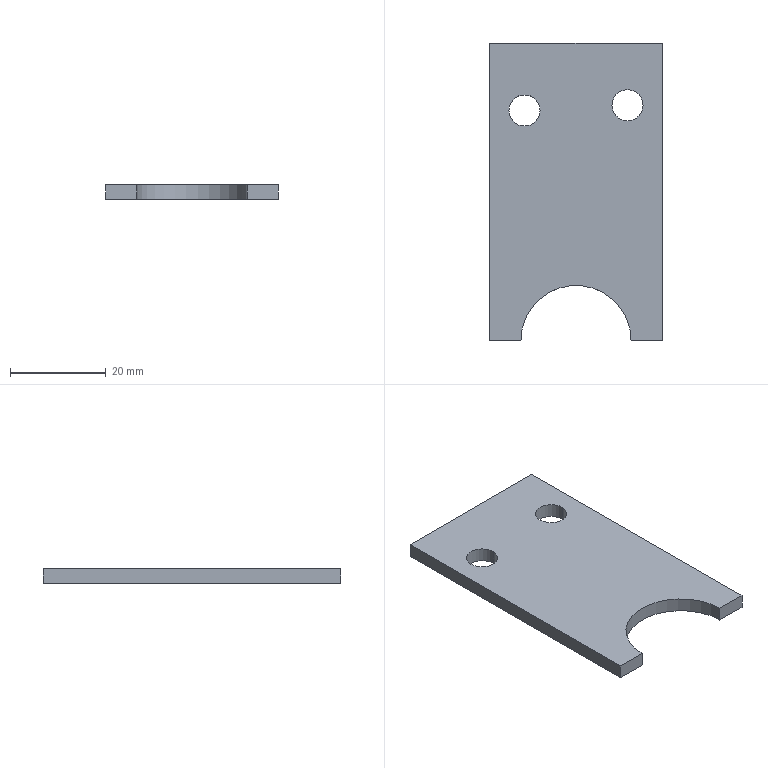Part | STEP file | 601-07-0070 | 1 solid | 12 faces | box 36 x 62 x 3 mm | volume 5874 mm3 | plane 7 | cylinder 5 | commonest cylinder face diameters 6.5 x4 23 x1
STEP:
#1=CARTESIAN_POINT('',(0.,0.,0.));
#2=DIRECTION('',(0.,0.,1.));
#3=DIRECTION('',(1.,0.,0.));
#4=AXIS2_PLACEMENT_3D('',#1,#2,#3);
#5=CARTESIAN_POINT('',(25.5,49.108,3.));
#6=VERTEX_POINT('',#5);
#7=CARTESIAN_POINT('',(25.5,49.108,0.));
#8=VERTEX_POINT('',#7);
#9=CARTESIAN_POINT('',(25.5,49.108,3.));
#10=DIRECTION('',(0.,0.,-1.));
#11=VECTOR('',#10,1.);
#12=LINE('',#9,#11);
#13=CARTESIAN_POINT('',(28.75,49.108,3.));
#14=DIRECTION('',(0.,0.,-1.));
#15=DIRECTION('',(-1.,0.,0.));
#16=AXIS2_PLACEMENT_3D('',#13,#14,#15);
#17=CYLINDRICAL_SURFACE('',#16,3.25);
#18=CARTESIAN_POINT('',(6.283,0.));
#19=DIRECTION('',(0.,1.));
#20=VECTOR('',#19,1.);
#21=LINE('',#18,#20);
#22=(GEOMETRIC_REPRESENTATION_CONTEXT(2)PARAMETRIC_REPRESENTATION_CONTEXT()REPRESENTATION_CONTEXT('',''));
#23=DEFINITIONAL_REPRESENTATION('',(#21),#22);
#24=PCURVE('',#17,#23);
#25=CARTESIAN_POINT('',(28.75,49.108,3.));
#26=DIRECTION('',(0.,0.,-1.));
#27=DIRECTION('',(-1.,0.,0.));
#28=AXIS2_PLACEMENT_3D('',#25,#26,#27);
#29=CYLINDRICAL_SURFACE('',#28,3.25);
#30=CARTESIAN_POINT('',(0.,0.));
#31=DIRECTION('',(0.,1.));
#32=VECTOR('',#31,1.);
#33=LINE('',#30,#32);
#34=(GEOMETRIC_REPRESENTATION_CONTEXT(2)PARAMETRIC_REPRESENTATION_CONTEXT()REPRESENTATION_CONTEXT('',''));
#35=DEFINITIONAL_REPRESENTATION('',(#33),#34);
#36=PCURVE('',#29,#35);
#37=SURFACE_CURVE('',#12,(#24,#36),.PCURVE_S1.);
#38=EDGE_CURVE('',#6,#8,#37,.T.);
#39=ORIENTED_EDGE('',*,*,#38,.T.);
#40=CARTESIAN_POINT('',(32.,49.108,0.));
#41=VERTEX_POINT('',#40);
#42=CARTESIAN_POINT('',(28.75,49.108,0.));
#43=DIRECTION('',(0.,0.,1.));
#44=DIRECTION('',(1.,0.,0.));
#45=AXIS2_PLACEMENT_3D('',#42,#43,#44);
#46=CIRCLE('',#45,3.25);
#47=CARTESIAN_POINT('',(9.425,3.));
#48=DIRECTION('',(-1.,0.));
#49=VECTOR('',#48,1.);
#50=LINE('',#47,#49);
#51=(GEOMETRIC_REPRESENTATION_CONTEXT(2)PARAMETRIC_REPRESENTATION_CONTEXT()REPRESENTATION_CONTEXT('',''));
#52=DEFINITIONAL_REPRESENTATION('',(#50),#51);
#53=PCURVE('',#17,#52);
#54=CARTESIAN_POINT('',(18.,0.,0.));
#55=DIRECTION('',(0.,0.,1.));
#56=DIRECTION('',(1.,0.,0.));
#57=AXIS2_PLACEMENT_3D('',#54,#55,#56);
#58=PLANE('',#57);
#59=CARTESIAN_POINT('',(10.75,49.108));
#60=DIRECTION('',(1.,0.));
#61=AXIS2_PLACEMENT_2D('',#59,#60);
#62=CIRCLE('',#61,3.25);
#63=(GEOMETRIC_REPRESENTATION_CONTEXT(2)PARAMETRIC_REPRESENTATION_CONTEXT()REPRESENTATION_CONTEXT('',''));
#64=DEFINITIONAL_REPRESENTATION('',(#62),#63);
#65=PCURVE('',#58,#64);
#66=SURFACE_CURVE('',#46,(#53,#65),.PCURVE_S1.);
#67=EDGE_CURVE('',#8,#41,#66,.T.);
#68=ORIENTED_EDGE('',*,*,#67,.T.);
#69=CARTESIAN_POINT('',(32.,49.108,3.));
#70=VERTEX_POINT('',#69);
#71=CARTESIAN_POINT('',(32.,49.108,3.));
#72=DIRECTION('',(0.,0.,-1.));
#73=VECTOR('',#72,1.);
#74=LINE('',#71,#73);
#75=CARTESIAN_POINT('',(3.142,0.));
#76=DIRECTION('',(0.,1.));
#77=VECTOR('',#76,1.);
#78=LINE('',#75,#77);
#79=(GEOMETRIC_REPRESENTATION_CONTEXT(2)PARAMETRIC_REPRESENTATION_CONTEXT()REPRESENTATION_CONTEXT('',''));
#80=DEFINITIONAL_REPRESENTATION('',(#78),#79);
#81=PCURVE('',#17,#80);
#82=CARTESIAN_POINT('',(3.142,0.));
#83=DIRECTION('',(0.,1.));
#84=VECTOR('',#83,1.);
#85=LINE('',#82,#84);
#86=(GEOMETRIC_REPRESENTATION_CONTEXT(2)PARAMETRIC_REPRESENTATION_CONTEXT()REPRESENTATION_CONTEXT('',''));
#87=DEFINITIONAL_REPRESENTATION('',(#85),#86);
#88=PCURVE('',#29,#87);
#89=SURFACE_CURVE('',#74,(#81,#88),.PCURVE_S1.);
#90=EDGE_CURVE('',#70,#41,#89,.T.);
#91=ORIENTED_EDGE('',*,*,#90,.F.);
#92=CARTESIAN_POINT('',(28.75,49.108,3.));
#93=DIRECTION('',(0.,0.,1.));
#94=DIRECTION('',(1.,0.,0.));
#95=AXIS2_PLACEMENT_3D('',#92,#93,#94);
#96=CIRCLE('',#95,3.25);
#97=CARTESIAN_POINT('',(9.425,0.));
#98=DIRECTION('',(-1.,0.));
#99=VECTOR('',#98,1.);
#100=LINE('',#97,#99);
#101=(GEOMETRIC_REPRESENTATION_CONTEXT(2)PARAMETRIC_REPRESENTATION_CONTEXT()REPRESENTATION_CONTEXT('',''));
#102=DEFINITIONAL_REPRESENTATION('',(#100),#101);
#103=PCURVE('',#17,#102);
#104=CARTESIAN_POINT('',(18.,0.,3.));
#105=DIRECTION('',(0.,0.,1.));
#106=DIRECTION('',(1.,0.,0.));
#107=AXIS2_PLACEMENT_3D('',#104,#105,#106);
#108=PLANE('',#107);
#109=CARTESIAN_POINT('',(10.75,49.108));
#110=DIRECTION('',(1.,0.));
#111=AXIS2_PLACEMENT_2D('',#109,#110);
#112=CIRCLE('',#111,3.25);
#113=(GEOMETRIC_REPRESENTATION_CONTEXT(2)PARAMETRIC_REPRESENTATION_CONTEXT()REPRESENTATION_CONTEXT('',''));
#114=DEFINITIONAL_REPRESENTATION('',(#112),#113);
#115=PCURVE('',#108,#114);
#116=SURFACE_CURVE('',#96,(#103,#115),.PCURVE_S1.);
#117=EDGE_CURVE('',#6,#70,#116,.T.);
#118=ORIENTED_EDGE('',*,*,#117,.F.);
#119=EDGE_LOOP('',(#39,#68,#91,#118));
#120=FACE_BOUND('',#119,.F.);
#121=ADVANCED_FACE('',(#120),#17,.F.);
#122=CARTESIAN_POINT('',(4.,48.,3.));
#123=VERTEX_POINT('',#122);
#124=CARTESIAN_POINT('',(4.,48.,0.));
#125=VERTEX_POINT('',#124);
#126=CARTESIAN_POINT('',(4.,48.,3.));
#127=DIRECTION('',(0.,0.,-1.));
#128=VECTOR('',#127,1.);
#129=LINE('',#126,#128);
#130=CARTESIAN_POINT('',(7.25,48.,3.));
#131=DIRECTION('',(0.,0.,-1.));
#132=DIRECTION('',(-1.,0.,0.));
#133=AXIS2_PLACEMENT_3D('',#130,#131,#132);
#134=CYLINDRICAL_SURFACE('',#133,3.25);
#135=CARTESIAN_POINT('',(6.283,0.));
#136=DIRECTION('',(0.,1.));
#137=VECTOR('',#136,1.);
#138=LINE('',#135,#137);
#139=(GEOMETRIC_REPRESENTATION_CONTEXT(2)PARAMETRIC_REPRESENTATION_CONTEXT()REPRESENTATION_CONTEXT('',''));
#140=DEFINITIONAL_REPRESENTATION('',(#138),#139);
#141=PCURVE('',#134,#140);
#142=CARTESIAN_POINT('',(7.25,48.,3.));
#143=DIRECTION('',(0.,0.,-1.));
#144=DIRECTION('',(-1.,0.,0.));
#145=AXIS2_PLACEMENT_3D('',#142,#143,#144);
#146=CYLINDRICAL_SURFACE('',#145,3.25);
#147=CARTESIAN_POINT('',(0.,0.));
#148=DIRECTION('',(0.,1.));
#149=VECTOR('',#148,1.);
#150=LINE('',#147,#149);
#151=(GEOMETRIC_REPRESENTATION_CONTEXT(2)PARAMETRIC_REPRESENTATION_CONTEXT()REPRESENTATION_CONTEXT('',''));
#152=DEFINITIONAL_REPRESENTATION('',(#150),#151);
#153=PCURVE('',#146,#152);
#154=SURFACE_CURVE('',#129,(#141,#153),.PCURVE_S1.);
#155=EDGE_CURVE('',#123,#125,#154,.T.);
#156=ORIENTED_EDGE('',*,*,#155,.T.);
#157=CARTESIAN_POINT('',(10.5,48.,0.));
#158=VERTEX_POINT('',#157);
#159=CARTESIAN_POINT('',(7.25,48.,0.));
#160=DIRECTION('',(0.,0.,1.));
#161=DIRECTION('',(1.,0.,0.));
#162=AXIS2_PLACEMENT_3D('',#159,#160,#161);
#163=CIRCLE('',#162,3.25);
#164=CARTESIAN_POINT('',(9.425,3.));
#165=DIRECTION('',(-1.,0.));
#166=VECTOR('',#165,1.);
#167=LINE('',#164,#166);
#168=(GEOMETRIC_REPRESENTATION_CONTEXT(2)PARAMETRIC_REPRESENTATION_CONTEXT()REPRESENTATION_CONTEXT('',''));
#169=DEFINITIONAL_REPRESENTATION('',(#167),#168);
#170=PCURVE('',#134,#169);
#171=CARTESIAN_POINT('',(-10.75,48.));
#172=DIRECTION('',(1.,0.));
#173=AXIS2_PLACEMENT_2D('',#171,#172);
#174=CIRCLE('',#173,3.25);
#175=(GEOMETRIC_REPRESENTATION_CONTEXT(2)PARAMETRIC_REPRESENTATION_CONTEXT()REPRESENTATION_CONTEXT('',''));
#176=DEFINITIONAL_REPRESENTATION('',(#174),#175);
#177=PCURVE('',#58,#176);
#178=SURFACE_CURVE('',#163,(#170,#177),.PCURVE_S1.);
#179=EDGE_CURVE('',#125,#158,#178,.T.);
#180=ORIENTED_EDGE('',*,*,#179,.T.);
#181=CARTESIAN_POINT('',(10.5,48.,3.));
#182=VERTEX_POINT('',#181);
#183=CARTESIAN_POINT('',(10.5,48.,3.));
#184=DIRECTION('',(0.,0.,-1.));
#185=VECTOR('',#184,1.);
#186=LINE('',#183,#185);
#187=CARTESIAN_POINT('',(3.142,0.));
#188=DIRECTION('',(0.,1.));
#189=VECTOR('',#188,1.);
#190=LINE('',#187,#189);
#191=(GEOMETRIC_REPRESENTATION_CONTEXT(2)PARAMETRIC_REPRESENTATION_CONTEXT()REPRESENTATION_CONTEXT('',''));
#192=DEFINITIONAL_REPRESENTATION('',(#190),#191);
#193=PCURVE('',#134,#192);
#194=CARTESIAN_POINT('',(3.142,0.));
#195=DIRECTION('',(0.,1.));
#196=VECTOR('',#195,1.);
#197=LINE('',#194,#196);
#198=(GEOMETRIC_REPRESENTATION_CONTEXT(2)PARAMETRIC_REPRESENTATION_CONTEXT()REPRESENTATION_CONTEXT('',''));
#199=DEFINITIONAL_REPRESENTATION('',(#197),#198);
#200=PCURVE('',#146,#199);
#201=SURFACE_CURVE('',#186,(#193,#200),.PCURVE_S1.);
#202=EDGE_CURVE('',#182,#158,#201,.T.);
#203=ORIENTED_EDGE('',*,*,#202,.F.);
#204=CARTESIAN_POINT('',(7.25,48.,3.));
#205=DIRECTION('',(0.,0.,1.));
#206=DIRECTION('',(1.,0.,0.));
#207=AXIS2_PLACEMENT_3D('',#204,#205,#206);
#208=CIRCLE('',#207,3.25);
#209=CARTESIAN_POINT('',(9.425,0.));
#210=DIRECTION('',(-1.,0.));
#211=VECTOR('',#210,1.);
#212=LINE('',#209,#211);
#213=(GEOMETRIC_REPRESENTATION_CONTEXT(2)PARAMETRIC_REPRESENTATION_CONTEXT()REPRESENTATION_CONTEXT('',''));
#214=DEFINITIONAL_REPRESENTATION('',(#212),#213);
#215=PCURVE('',#134,#214);
#216=CARTESIAN_POINT('',(-10.75,48.));
#217=DIRECTION('',(1.,0.));
#218=AXIS2_PLACEMENT_2D('',#216,#217);
#219=CIRCLE('',#218,3.25);
#220=(GEOMETRIC_REPRESENTATION_CONTEXT(2)PARAMETRIC_REPRESENTATION_CONTEXT()REPRESENTATION_CONTEXT('',''));
#221=DEFINITIONAL_REPRESENTATION('',(#219),#220);
#222=PCURVE('',#108,#221);
#223=SURFACE_CURVE('',#208,(#215,#222),.PCURVE_S1.);
#224=EDGE_CURVE('',#123,#182,#223,.T.);
#225=ORIENTED_EDGE('',*,*,#224,.F.);
#226=EDGE_LOOP('',(#156,#180,#203,#225));
#227=FACE_BOUND('',#226,.F.);
#228=ADVANCED_FACE('',(#227),#134,.F.);
#229=ORIENTED_EDGE('',*,*,#224,.F.);
#230=CARTESIAN_POINT('',(7.25,48.,3.));
#231=DIRECTION('',(0.,0.,1.));
#232=DIRECTION('',(1.,0.,0.));
#233=AXIS2_PLACEMENT_3D('',#230,#231,#232);
#234=CIRCLE('',#233,3.25);
#235=CARTESIAN_POINT('',(-10.75,48.));
#236=DIRECTION('',(1.,0.));
#237=AXIS2_PLACEMENT_2D('',#235,#236);
#238=CIRCLE('',#237,3.25);
#239=(GEOMETRIC_REPRESENTATION_CONTEXT(2)PARAMETRIC_REPRESENTATION_CONTEXT()REPRESENTATION_CONTEXT('',''));
#240=DEFINITIONAL_REPRESENTATION('',(#238),#239);
#241=PCURVE('',#108,#240);
#242=CARTESIAN_POINT('',(3.142,0.));
#243=DIRECTION('',(-1.,0.));
#244=VECTOR('',#243,1.);
#245=LINE('',#242,#244);
#246=(GEOMETRIC_REPRESENTATION_CONTEXT(2)PARAMETRIC_REPRESENTATION_CONTEXT()REPRESENTATION_CONTEXT('',''));
#247=DEFINITIONAL_REPRESENTATION('',(#245),#246);
#248=PCURVE('',#146,#247);
#249=SURFACE_CURVE('',#234,(#241,#248),.PCURVE_S1.);
#250=EDGE_CURVE('',#182,#123,#249,.T.);
#251=ORIENTED_EDGE('',*,*,#250,.F.);
#252=EDGE_LOOP('',(#229,#251));
#253=FACE_BOUND('',#252,.T.);
#254=CARTESIAN_POINT('',(0.,62.,3.));
#255=VERTEX_POINT('',#254);
#256=CARTESIAN_POINT('',(0.,0.,3.));
#257=VERTEX_POINT('',#256);
#258=CARTESIAN_POINT('',(0.,0.,3.));
#259=DIRECTION('',(0.,-1.,0.));
#260=VECTOR('',#259,1.);
#261=LINE('',#258,#260);
#262=CARTESIAN_POINT('',(-18.,0.));
#263=DIRECTION('',(0.,-1.));
#264=VECTOR('',#263,1.);
#265=LINE('',#262,#264);
#266=(GEOMETRIC_REPRESENTATION_CONTEXT(2)PARAMETRIC_REPRESENTATION_CONTEXT()REPRESENTATION_CONTEXT('',''));
#267=DEFINITIONAL_REPRESENTATION('',(#265),#266);
#268=PCURVE('',#108,#267);
#269=CARTESIAN_POINT('',(0.,0.,3.));
#270=DIRECTION('',(1.,0.,0.));
#271=DIRECTION('',(0.,1.,0.));
#272=AXIS2_PLACEMENT_3D('',#269,#270,#271);
#273=PLANE('',#272);
#274=CARTESIAN_POINT('',(0.,0.));
#275=DIRECTION('',(-1.,0.));
#276=VECTOR('',#275,1.);
#277=LINE('',#274,#276);
#278=(GEOMETRIC_REPRESENTATION_CONTEXT(2)PARAMETRIC_REPRESENTATION_CONTEXT()REPRESENTATION_CONTEXT('',''));
#279=DEFINITIONAL_REPRESENTATION('',(#277),#278);
#280=PCURVE('',#273,#279);
#281=SURFACE_CURVE('',#261,(#268,#280),.PCURVE_S1.);
#282=EDGE_CURVE('',#255,#257,#281,.T.);
#283=ORIENTED_EDGE('',*,*,#282,.T.);
#284=CARTESIAN_POINT('',(6.5,0.,3.));
#285=VERTEX_POINT('',#284);
#286=CARTESIAN_POINT('',(0.,0.,3.));
#287=DIRECTION('',(1.,0.,0.));
#288=VECTOR('',#287,1.);
#289=LINE('',#286,#288);
#290=CARTESIAN_POINT('',(-18.,0.));
#291=DIRECTION('',(1.,0.));
#292=VECTOR('',#291,1.);
#293=LINE('',#290,#292);
#294=(GEOMETRIC_REPRESENTATION_CONTEXT(2)PARAMETRIC_REPRESENTATION_CONTEXT()REPRESENTATION_CONTEXT('',''));
#295=DEFINITIONAL_REPRESENTATION('',(#293),#294);
#296=PCURVE('',#108,#295);
#297=CARTESIAN_POINT('',(0.,0.,3.));
#298=DIRECTION('',(0.,1.,0.));
#299=DIRECTION('',(0.,0.,1.));
#300=AXIS2_PLACEMENT_3D('',#297,#298,#299);
#301=PLANE('',#300);
#302=CARTESIAN_POINT('',(0.,0.));
#303=DIRECTION('',(0.,1.));
#304=VECTOR('',#303,1.);
#305=LINE('',#302,#304);
#306=(GEOMETRIC_REPRESENTATION_CONTEXT(2)PARAMETRIC_REPRESENTATION_CONTEXT()REPRESENTATION_CONTEXT('',''));
#307=DEFINITIONAL_REPRESENTATION('',(#305),#306);
#308=PCURVE('',#301,#307);
#309=SURFACE_CURVE('',#289,(#296,#308),.PCURVE_S1.);
#310=EDGE_CURVE('',#257,#285,#309,.T.);
#311=ORIENTED_EDGE('',*,*,#310,.T.);
#312=CARTESIAN_POINT('',(29.5,0.,3.));
#313=VERTEX_POINT('',#312);
#314=CARTESIAN_POINT('',(18.,0.,3.));
#315=DIRECTION('',(0.,0.,-1.));
#316=DIRECTION('',(1.,0.,0.));
#317=AXIS2_PLACEMENT_3D('',#314,#315,#316);
#318=CIRCLE('',#317,11.5);
#319=CARTESIAN_POINT('',(11.5,0.));
#320=CARTESIAN_POINT('',(11.5,-19.919));
#321=CARTESIAN_POINT('',(-5.75,-9.959));
#322=CARTESIAN_POINT('',(-23.,0.));
#323=CARTESIAN_POINT('',(-5.75,9.959));
#324=CARTESIAN_POINT('',(11.5,19.919));
#325=CARTESIAN_POINT('',(11.5,0.));
#326=(BOUNDED_CURVE()B_SPLINE_CURVE(2,(#319,#320,#321,#322,#323,#324,#325),.UNSPECIFIED.,.T.,.F.)B_SPLINE_CURVE_WITH_KNOTS((1,2,2,2,2,1),(-2.094,0.,2.094,4.189,6.283,8.378),.UNSPECIFIED.)CURVE()GEOMETRIC_REPRESENTATION_ITEM()RATIONAL_B_SPLINE_CURVE((1.,0.5,1.,0.5,1.,0.5,1.))REPRESENTATION_ITEM(''));
#327=(GEOMETRIC_REPRESENTATION_CONTEXT(2)PARAMETRIC_REPRESENTATION_CONTEXT()REPRESENTATION_CONTEXT('',''));
#328=DEFINITIONAL_REPRESENTATION('',(#326),#327);
#329=PCURVE('',#108,#328);
#330=CARTESIAN_POINT('',(18.,0.,3.));
#331=DIRECTION('',(0.,0.,-1.));
#332=DIRECTION('',(-1.,0.,0.));
#333=AXIS2_PLACEMENT_3D('',#330,#331,#332);
#334=CYLINDRICAL_SURFACE('',#333,11.5);
#335=CARTESIAN_POINT('',(-3.142,0.));
#336=DIRECTION('',(1.,0.));
#337=VECTOR('',#336,1.);
#338=LINE('',#335,#337);
#339=(GEOMETRIC_REPRESENTATION_CONTEXT(2)PARAMETRIC_REPRESENTATION_CONTEXT()REPRESENTATION_CONTEXT('',''));
#340=DEFINITIONAL_REPRESENTATION('',(#338),#339);
#341=PCURVE('',#334,#340);
#342=SURFACE_CURVE('',#318,(#329,#341),.PCURVE_S1.);
#343=EDGE_CURVE('',#285,#313,#342,.T.);
#344=ORIENTED_EDGE('',*,*,#343,.T.);
#345=CARTESIAN_POINT('',(36.,0.,3.));
#346=VERTEX_POINT('',#345);
#347=CARTESIAN_POINT('',(29.5,0.,3.));
#348=DIRECTION('',(1.,0.,0.));
#349=VECTOR('',#348,1.);
#350=LINE('',#347,#349);
#351=CARTESIAN_POINT('',(11.5,0.));
#352=DIRECTION('',(1.,0.));
#353=VECTOR('',#352,1.);
#354=LINE('',#351,#353);
#355=(GEOMETRIC_REPRESENTATION_CONTEXT(2)PARAMETRIC_REPRESENTATION_CONTEXT()REPRESENTATION_CONTEXT('',''));
#356=DEFINITIONAL_REPRESENTATION('',(#354),#355);
#357=PCURVE('',#108,#356);
#358=CARTESIAN_POINT('',(29.5,0.,3.));
#359=DIRECTION('',(0.,1.,0.));
#360=DIRECTION('',(0.,0.,1.));
#361=AXIS2_PLACEMENT_3D('',#358,#359,#360);
#362=PLANE('',#361);
#363=CARTESIAN_POINT('',(0.,0.));
#364=DIRECTION('',(0.,1.));
#365=VECTOR('',#364,1.);
#366=LINE('',#363,#365);
#367=(GEOMETRIC_REPRESENTATION_CONTEXT(2)PARAMETRIC_REPRESENTATION_CONTEXT()REPRESENTATION_CONTEXT('',''));
#368=DEFINITIONAL_REPRESENTATION('',(#366),#367);
#369=PCURVE('',#362,#368);
#370=SURFACE_CURVE('',#350,(#357,#369),.PCURVE_S1.);
#371=EDGE_CURVE('',#313,#346,#370,.T.);
#372=ORIENTED_EDGE('',*,*,#371,.T.);
#373=CARTESIAN_POINT('',(36.,62.,3.));
#374=VERTEX_POINT('',#373);
#375=CARTESIAN_POINT('',(36.,0.,3.));
#376=DIRECTION('',(0.,1.,0.));
#377=VECTOR('',#376,1.);
#378=LINE('',#375,#377);
#379=CARTESIAN_POINT('',(18.,0.));
#380=DIRECTION('',(0.,1.));
#381=VECTOR('',#380,1.);
#382=LINE('',#379,#381);
#383=(GEOMETRIC_REPRESENTATION_CONTEXT(2)PARAMETRIC_REPRESENTATION_CONTEXT()REPRESENTATION_CONTEXT('',''));
#384=DEFINITIONAL_REPRESENTATION('',(#382),#383);
#385=PCURVE('',#108,#384);
#386=CARTESIAN_POINT('',(36.,0.,3.));
#387=DIRECTION('',(-1.,0.,0.));
#388=DIRECTION('',(0.,-1.,0.));
#389=AXIS2_PLACEMENT_3D('',#386,#387,#388);
#390=PLANE('',#389);
#391=CARTESIAN_POINT('',(0.,0.));
#392=DIRECTION('',(-1.,0.));
#393=VECTOR('',#392,1.);
#394=LINE('',#391,#393);
#395=(GEOMETRIC_REPRESENTATION_CONTEXT(2)PARAMETRIC_REPRESENTATION_CONTEXT()REPRESENTATION_CONTEXT('',''));
#396=DEFINITIONAL_REPRESENTATION('',(#394),#395);
#397=PCURVE('',#390,#396);
#398=SURFACE_CURVE('',#378,(#385,#397),.PCURVE_S1.);
#399=EDGE_CURVE('',#346,#374,#398,.T.);
#400=ORIENTED_EDGE('',*,*,#399,.T.);
#401=CARTESIAN_POINT('',(0.,62.,3.));
#402=DIRECTION('',(-1.,0.,0.));
#403=VECTOR('',#402,1.);
#404=LINE('',#401,#403);
#405=CARTESIAN_POINT('',(-18.,62.));
#406=DIRECTION('',(-1.,0.));
#407=VECTOR('',#406,1.);
#408=LINE('',#405,#407);
#409=(GEOMETRIC_REPRESENTATION_CONTEXT(2)PARAMETRIC_REPRESENTATION_CONTEXT()REPRESENTATION_CONTEXT('',''));
#410=DEFINITIONAL_REPRESENTATION('',(#408),#409);
#411=PCURVE('',#108,#410);
#412=CARTESIAN_POINT('',(0.,62.,3.));
#413=DIRECTION('',(0.,-1.,0.));
#414=DIRECTION('',(0.,0.,-1.));
#415=AXIS2_PLACEMENT_3D('',#412,#413,#414);
#416=PLANE('',#415);
#417=CARTESIAN_POINT('',(0.,0.));
#418=DIRECTION('',(0.,-1.));
#419=VECTOR('',#418,1.);
#420=LINE('',#417,#419);
#421=(GEOMETRIC_REPRESENTATION_CONTEXT(2)PARAMETRIC_REPRESENTATION_CONTEXT()REPRESENTATION_CONTEXT('',''));
#422=DEFINITIONAL_REPRESENTATION('',(#420),#421);
#423=PCURVE('',#416,#422);
#424=SURFACE_CURVE('',#404,(#411,#423),.PCURVE_S1.);
#425=EDGE_CURVE('',#374,#255,#424,.T.);
#426=ORIENTED_EDGE('',*,*,#425,.T.);
#427=EDGE_LOOP('',(#283,#311,#344,#372,#400,#426));
#428=FACE_BOUND('',#427,.T.);
#429=ORIENTED_EDGE('',*,*,#117,.F.);
#430=CARTESIAN_POINT('',(28.75,49.108,3.));
#431=DIRECTION('',(0.,0.,1.));
#432=DIRECTION('',(1.,0.,0.));
#433=AXIS2_PLACEMENT_3D('',#430,#431,#432);
#434=CIRCLE('',#433,3.25);
#435=CARTESIAN_POINT('',(10.75,49.108));
#436=DIRECTION('',(1.,0.));
#437=AXIS2_PLACEMENT_2D('',#435,#436);
#438=CIRCLE('',#437,3.25);
#439=(GEOMETRIC_REPRESENTATION_CONTEXT(2)PARAMETRIC_REPRESENTATION_CONTEXT()REPRESENTATION_CONTEXT('',''));
#440=DEFINITIONAL_REPRESENTATION('',(#438),#439);
#441=PCURVE('',#108,#440);
#442=CARTESIAN_POINT('',(3.142,0.));
#443=DIRECTION('',(-1.,0.));
#444=VECTOR('',#443,1.);
#445=LINE('',#442,#444);
#446=(GEOMETRIC_REPRESENTATION_CONTEXT(2)PARAMETRIC_REPRESENTATION_CONTEXT()REPRESENTATION_CONTEXT('',''));
#447=DEFINITIONAL_REPRESENTATION('',(#445),#446);
#448=PCURVE('',#29,#447);
#449=SURFACE_CURVE('',#434,(#441,#448),.PCURVE_S1.);
#450=EDGE_CURVE('',#70,#6,#449,.T.);
#451=ORIENTED_EDGE('',*,*,#450,.F.);
#452=EDGE_LOOP('',(#429,#451));
#453=FACE_BOUND('',#452,.T.);
#454=ADVANCED_FACE('',(#253,#428,#453),#108,.T.);
#455=ORIENTED_EDGE('',*,*,#179,.T.);
#456=CARTESIAN_POINT('',(7.25,48.,0.));
#457=DIRECTION('',(0.,0.,1.));
#458=DIRECTION('',(1.,0.,0.));
#459=AXIS2_PLACEMENT_3D('',#456,#457,#458);
#460=CIRCLE('',#459,3.25);
#461=CARTESIAN_POINT('',(-10.75,48.));
#462=DIRECTION('',(1.,0.));
#463=AXIS2_PLACEMENT_2D('',#461,#462);
#464=CIRCLE('',#463,3.25);
#465=(GEOMETRIC_REPRESENTATION_CONTEXT(2)PARAMETRIC_REPRESENTATION_CONTEXT()REPRESENTATION_CONTEXT('',''));
#466=DEFINITIONAL_REPRESENTATION('',(#464),#465);
#467=PCURVE('',#58,#466);
#468=CARTESIAN_POINT('',(3.142,3.));
#469=DIRECTION('',(-1.,0.));
#470=VECTOR('',#469,1.);
#471=LINE('',#468,#470);
#472=(GEOMETRIC_REPRESENTATION_CONTEXT(2)PARAMETRIC_REPRESENTATION_CONTEXT()REPRESENTATION_CONTEXT('',''));
#473=DEFINITIONAL_REPRESENTATION('',(#471),#472);
#474=PCURVE('',#146,#473);
#475=SURFACE_CURVE('',#460,(#467,#474),.PCURVE_S1.);
#476=EDGE_CURVE('',#158,#125,#475,.T.);
#477=ORIENTED_EDGE('',*,*,#476,.T.);
#478=EDGE_LOOP('',(#455,#477));
#479=FACE_BOUND('',#478,.T.);
#480=CARTESIAN_POINT('',(0.,62.,0.));
#481=VERTEX_POINT('',#480);
#482=CARTESIAN_POINT('',(0.,0.,0.));
#483=VERTEX_POINT('',#482);
#484=CARTESIAN_POINT('',(0.,0.,0.));
#485=DIRECTION('',(0.,-1.,0.));
#486=VECTOR('',#485,1.);
#487=LINE('',#484,#486);
#488=CARTESIAN_POINT('',(-18.,0.));
#489=DIRECTION('',(0.,-1.));
#490=VECTOR('',#489,1.);
#491=LINE('',#488,#490);
#492=(GEOMETRIC_REPRESENTATION_CONTEXT(2)PARAMETRIC_REPRESENTATION_CONTEXT()REPRESENTATION_CONTEXT('',''));
#493=DEFINITIONAL_REPRESENTATION('',(#491),#492);
#494=PCURVE('',#58,#493);
#495=CARTESIAN_POINT('',(0.,-3.));
#496=DIRECTION('',(-1.,0.));
#497=VECTOR('',#496,1.);
#498=LINE('',#495,#497);
#499=(GEOMETRIC_REPRESENTATION_CONTEXT(2)PARAMETRIC_REPRESENTATION_CONTEXT()REPRESENTATION_CONTEXT('',''));
#500=DEFINITIONAL_REPRESENTATION('',(#498),#499);
#501=PCURVE('',#273,#500);
#502=SURFACE_CURVE('',#487,(#494,#501),.PCURVE_S1.);
#503=EDGE_CURVE('',#481,#483,#502,.T.);
#504=ORIENTED_EDGE('',*,*,#503,.F.);
#505=CARTESIAN_POINT('',(36.,62.,0.));
#506=VERTEX_POINT('',#505);
#507=CARTESIAN_POINT('',(0.,62.,0.));
#508=DIRECTION('',(-1.,0.,0.));
#509=VECTOR('',#508,1.);
#510=LINE('',#507,#509);
#511=CARTESIAN_POINT('',(-18.,62.));
#512=DIRECTION('',(-1.,0.));
#513=VECTOR('',#512,1.);
#514=LINE('',#511,#513);
#515=(GEOMETRIC_REPRESENTATION_CONTEXT(2)PARAMETRIC_REPRESENTATION_CONTEXT()REPRESENTATION_CONTEXT('',''));
#516=DEFINITIONAL_REPRESENTATION('',(#514),#515);
#517=PCURVE('',#58,#516);
#518=CARTESIAN_POINT('',(3.,0.));
#519=DIRECTION('',(0.,-1.));
#520=VECTOR('',#519,1.);
#521=LINE('',#518,#520);
#522=(GEOMETRIC_REPRESENTATION_CONTEXT(2)PARAMETRIC_REPRESENTATION_CONTEXT()REPRESENTATION_CONTEXT('',''));
#523=DEFINITIONAL_REPRESENTATION('',(#521),#522);
#524=PCURVE('',#416,#523);
#525=SURFACE_CURVE('',#510,(#517,#524),.PCURVE_S1.);
#526=EDGE_CURVE('',#506,#481,#525,.T.);
#527=ORIENTED_EDGE('',*,*,#526,.F.);
#528=CARTESIAN_POINT('',(36.,0.,0.));
#529=VERTEX_POINT('',#528);
#530=CARTESIAN_POINT('',(36.,0.,0.));
#531=DIRECTION('',(0.,1.,0.));
#532=VECTOR('',#531,1.);
#533=LINE('',#530,#532);
#534=CARTESIAN_POINT('',(18.,0.));
#535=DIRECTION('',(0.,1.));
#536=VECTOR('',#535,1.);
#537=LINE('',#534,#536);
#538=(GEOMETRIC_REPRESENTATION_CONTEXT(2)PARAMETRIC_REPRESENTATION_CONTEXT()REPRESENTATION_CONTEXT('',''));
#539=DEFINITIONAL_REPRESENTATION('',(#537),#538);
#540=PCURVE('',#58,#539);
#541=CARTESIAN_POINT('',(0.,-3.));
#542=DIRECTION('',(-1.,0.));
#543=VECTOR('',#542,1.);
#544=LINE('',#541,#543);
#545=(GEOMETRIC_REPRESENTATION_CONTEXT(2)PARAMETRIC_REPRESENTATION_CONTEXT()REPRESENTATION_CONTEXT('',''));
#546=DEFINITIONAL_REPRESENTATION('',(#544),#545);
#547=PCURVE('',#390,#546);
#548=SURFACE_CURVE('',#533,(#540,#547),.PCURVE_S1.);
#549=EDGE_CURVE('',#529,#506,#548,.T.);
#550=ORIENTED_EDGE('',*,*,#549,.F.);
#551=CARTESIAN_POINT('',(29.5,0.,0.));
#552=VERTEX_POINT('',#551);
#553=CARTESIAN_POINT('',(29.5,0.,0.));
#554=DIRECTION('',(1.,0.,0.));
#555=VECTOR('',#554,1.);
#556=LINE('',#553,#555);
#557=CARTESIAN_POINT('',(11.5,0.));
#558=DIRECTION('',(1.,0.));
#559=VECTOR('',#558,1.);
#560=LINE('',#557,#559);
#561=(GEOMETRIC_REPRESENTATION_CONTEXT(2)PARAMETRIC_REPRESENTATION_CONTEXT()REPRESENTATION_CONTEXT('',''));
#562=DEFINITIONAL_REPRESENTATION('',(#560),#561);
#563=PCURVE('',#58,#562);
#564=CARTESIAN_POINT('',(-3.,0.));
#565=DIRECTION('',(0.,1.));
#566=VECTOR('',#565,1.);
#567=LINE('',#564,#566);
#568=(GEOMETRIC_REPRESENTATION_CONTEXT(2)PARAMETRIC_REPRESENTATION_CONTEXT()REPRESENTATION_CONTEXT('',''));
#569=DEFINITIONAL_REPRESENTATION('',(#567),#568);
#570=PCURVE('',#362,#569);
#571=SURFACE_CURVE('',#556,(#563,#570),.PCURVE_S1.);
#572=EDGE_CURVE('',#552,#529,#571,.T.);
#573=ORIENTED_EDGE('',*,*,#572,.F.);
#574=CARTESIAN_POINT('',(6.5,0.,0.));
#575=VERTEX_POINT('',#574);
#576=CARTESIAN_POINT('',(18.,0.,0.));
#577=DIRECTION('',(0.,0.,-1.));
#578=DIRECTION('',(1.,0.,0.));
#579=AXIS2_PLACEMENT_3D('',#576,#577,#578);
#580=CIRCLE('',#579,11.5);
#581=CARTESIAN_POINT('',(11.5,0.));
#582=CARTESIAN_POINT('',(11.5,-19.919));
#583=CARTESIAN_POINT('',(-5.75,-9.959));
#584=CARTESIAN_POINT('',(-23.,0.));
#585=CARTESIAN_POINT('',(-5.75,9.959));
#586=CARTESIAN_POINT('',(11.5,19.919));
#587=CARTESIAN_POINT('',(11.5,0.));
#588=(BOUNDED_CURVE()B_SPLINE_CURVE(2,(#581,#582,#583,#584,#585,#586,#587),.UNSPECIFIED.,.T.,.F.)B_SPLINE_CURVE_WITH_KNOTS((1,2,2,2,2,1),(-2.094,0.,2.094,4.189,6.283,8.378),.UNSPECIFIED.)CURVE()GEOMETRIC_REPRESENTATION_ITEM()RATIONAL_B_SPLINE_CURVE((1.,0.5,1.,0.5,1.,0.5,1.))REPRESENTATION_ITEM(''));
#589=(GEOMETRIC_REPRESENTATION_CONTEXT(2)PARAMETRIC_REPRESENTATION_CONTEXT()REPRESENTATION_CONTEXT('',''));
#590=DEFINITIONAL_REPRESENTATION('',(#588),#589);
#591=PCURVE('',#58,#590);
#592=CARTESIAN_POINT('',(-3.142,3.));
#593=DIRECTION('',(1.,0.));
#594=VECTOR('',#593,1.);
#595=LINE('',#592,#594);
#596=(GEOMETRIC_REPRESENTATION_CONTEXT(2)PARAMETRIC_REPRESENTATION_CONTEXT()REPRESENTATION_CONTEXT('',''));
#597=DEFINITIONAL_REPRESENTATION('',(#595),#596);
#598=PCURVE('',#334,#597);
#599=SURFACE_CURVE('',#580,(#591,#598),.PCURVE_S1.);
#600=EDGE_CURVE('',#575,#552,#599,.T.);
#601=ORIENTED_EDGE('',*,*,#600,.F.);
#602=CARTESIAN_POINT('',(0.,0.,0.));
#603=DIRECTION('',(1.,0.,0.));
#604=VECTOR('',#603,1.);
#605=LINE('',#602,#604);
#606=CARTESIAN_POINT('',(-18.,0.));
#607=DIRECTION('',(1.,0.));
#608=VECTOR('',#607,1.);
#609=LINE('',#606,#608);
#610=(GEOMETRIC_REPRESENTATION_CONTEXT(2)PARAMETRIC_REPRESENTATION_CONTEXT()REPRESENTATION_CONTEXT('',''));
#611=DEFINITIONAL_REPRESENTATION('',(#609),#610);
#612=PCURVE('',#58,#611);
#613=CARTESIAN_POINT('',(-3.,0.));
#614=DIRECTION('',(0.,1.));
#615=VECTOR('',#614,1.);
#616=LINE('',#613,#615);
#617=(GEOMETRIC_REPRESENTATION_CONTEXT(2)PARAMETRIC_REPRESENTATION_CONTEXT()REPRESENTATION_CONTEXT('',''));
#618=DEFINITIONAL_REPRESENTATION('',(#616),#617);
#619=PCURVE('',#301,#618);
#620=SURFACE_CURVE('',#605,(#612,#619),.PCURVE_S1.);
#621=EDGE_CURVE('',#483,#575,#620,.T.);
#622=ORIENTED_EDGE('',*,*,#621,.F.);
#623=EDGE_LOOP('',(#504,#527,#550,#573,#601,#622));
#624=FACE_BOUND('',#623,.T.);
#625=ORIENTED_EDGE('',*,*,#67,.T.);
#626=CARTESIAN_POINT('',(28.75,49.108,0.));
#627=DIRECTION('',(0.,0.,1.));
#628=DIRECTION('',(1.,0.,0.));
#629=AXIS2_PLACEMENT_3D('',#626,#627,#628);
#630=CIRCLE('',#629,3.25);
#631=CARTESIAN_POINT('',(10.75,49.108));
#632=DIRECTION('',(1.,0.));
#633=AXIS2_PLACEMENT_2D('',#631,#632);
#634=CIRCLE('',#633,3.25);
#635=(GEOMETRIC_REPRESENTATION_CONTEXT(2)PARAMETRIC_REPRESENTATION_CONTEXT()REPRESENTATION_CONTEXT('',''));
#636=DEFINITIONAL_REPRESENTATION('',(#634),#635);
#637=PCURVE('',#58,#636);
#638=CARTESIAN_POINT('',(3.142,3.));
#639=DIRECTION('',(-1.,0.));
#640=VECTOR('',#639,1.);
#641=LINE('',#638,#640);
#642=(GEOMETRIC_REPRESENTATION_CONTEXT(2)PARAMETRIC_REPRESENTATION_CONTEXT()REPRESENTATION_CONTEXT('',''));
#643=DEFINITIONAL_REPRESENTATION('',(#641),#642);
#644=PCURVE('',#29,#643);
#645=SURFACE_CURVE('',#630,(#637,#644),.PCURVE_S1.);
#646=EDGE_CURVE('',#41,#8,#645,.T.);
#647=ORIENTED_EDGE('',*,*,#646,.T.);
#648=EDGE_LOOP('',(#625,#647));
#649=FACE_BOUND('',#648,.T.);
#650=ADVANCED_FACE('',(#479,#624,#649),#58,.F.);
#651=ORIENTED_EDGE('',*,*,#503,.T.);
#652=CARTESIAN_POINT('',(0.,0.,3.));
#653=DIRECTION('',(0.,0.,-1.));
#654=VECTOR('',#653,1.);
#655=LINE('',#652,#654);
#656=CARTESIAN_POINT('',(0.,0.));
#657=DIRECTION('',(0.,-1.));
#658=VECTOR('',#657,1.);
#659=LINE('',#656,#658);
#660=(GEOMETRIC_REPRESENTATION_CONTEXT(2)PARAMETRIC_REPRESENTATION_CONTEXT()REPRESENTATION_CONTEXT('',''));
#661=DEFINITIONAL_REPRESENTATION('',(#659),#660);
#662=PCURVE('',#273,#661);
#663=CARTESIAN_POINT('',(0.,0.));
#664=DIRECTION('',(-1.,0.));
#665=VECTOR('',#664,1.);
#666=LINE('',#663,#665);
#667=(GEOMETRIC_REPRESENTATION_CONTEXT(2)PARAMETRIC_REPRESENTATION_CONTEXT()REPRESENTATION_CONTEXT('',''));
#668=DEFINITIONAL_REPRESENTATION('',(#666),#667);
#669=PCURVE('',#301,#668);
#670=SURFACE_CURVE('',#655,(#662,#669),.PCURVE_S1.);
#671=EDGE_CURVE('',#257,#483,#670,.T.);
#672=ORIENTED_EDGE('',*,*,#671,.F.);
#673=ORIENTED_EDGE('',*,*,#282,.F.);
#674=CARTESIAN_POINT('',(0.,62.,3.));
#675=DIRECTION('',(0.,0.,-1.));
#676=VECTOR('',#675,1.);
#677=LINE('',#674,#676);
#678=CARTESIAN_POINT('',(62.,0.));
#679=DIRECTION('',(0.,-1.));
#680=VECTOR('',#679,1.);
#681=LINE('',#678,#680);
#682=(GEOMETRIC_REPRESENTATION_CONTEXT(2)PARAMETRIC_REPRESENTATION_CONTEXT()REPRESENTATION_CONTEXT('',''));
#683=DEFINITIONAL_REPRESENTATION('',(#681),#682);
#684=PCURVE('',#273,#683);
#685=CARTESIAN_POINT('',(0.,0.));
#686=DIRECTION('',(1.,0.));
#687=VECTOR('',#686,1.);
#688=LINE('',#685,#687);
#689=(GEOMETRIC_REPRESENTATION_CONTEXT(2)PARAMETRIC_REPRESENTATION_CONTEXT()REPRESENTATION_CONTEXT('',''));
#690=DEFINITIONAL_REPRESENTATION('',(#688),#689);
#691=PCURVE('',#416,#690);
#692=SURFACE_CURVE('',#677,(#684,#691),.PCURVE_S1.);
#693=EDGE_CURVE('',#255,#481,#692,.T.);
#694=ORIENTED_EDGE('',*,*,#693,.T.);
#695=EDGE_LOOP('',(#651,#672,#673,#694));
#696=FACE_BOUND('',#695,.T.);
#697=ADVANCED_FACE('',(#696),#273,.F.);
#698=ORIENTED_EDGE('',*,*,#621,.T.);
#699=CARTESIAN_POINT('',(6.5,0.,3.));
#700=DIRECTION('',(0.,0.,-1.));
#701=VECTOR('',#700,1.);
#702=LINE('',#699,#701);
#703=CARTESIAN_POINT('',(0.,6.5));
#704=DIRECTION('',(-1.,0.));
#705=VECTOR('',#704,1.);
#706=LINE('',#703,#705);
#707=(GEOMETRIC_REPRESENTATION_CONTEXT(2)PARAMETRIC_REPRESENTATION_CONTEXT()REPRESENTATION_CONTEXT('',''));
#708=DEFINITIONAL_REPRESENTATION('',(#706),#707);
#709=PCURVE('',#301,#708);
#710=CARTESIAN_POINT('',(0.,0.));
#711=DIRECTION('',(0.,1.));
#712=VECTOR('',#711,1.);
#713=LINE('',#710,#712);
#714=(GEOMETRIC_REPRESENTATION_CONTEXT(2)PARAMETRIC_REPRESENTATION_CONTEXT()REPRESENTATION_CONTEXT('',''));
#715=DEFINITIONAL_REPRESENTATION('',(#713),#714);
#716=PCURVE('',#334,#715);
#717=SURFACE_CURVE('',#702,(#709,#716),.PCURVE_S1.);
#718=EDGE_CURVE('',#285,#575,#717,.T.);
#719=ORIENTED_EDGE('',*,*,#718,.F.);
#720=ORIENTED_EDGE('',*,*,#310,.F.);
#721=ORIENTED_EDGE('',*,*,#671,.T.);
#722=EDGE_LOOP('',(#698,#719,#720,#721));
#723=FACE_BOUND('',#722,.T.);
#724=ADVANCED_FACE('',(#723),#301,.F.);
#725=ORIENTED_EDGE('',*,*,#718,.F.);
#726=ORIENTED_EDGE('',*,*,#343,.T.);
#727=CARTESIAN_POINT('',(29.5,0.,3.));
#728=DIRECTION('',(0.,0.,-1.));
#729=VECTOR('',#728,1.);
#730=LINE('',#727,#729);
#731=CARTESIAN_POINT('',(3.142,0.));
#732=DIRECTION('',(0.,1.));
#733=VECTOR('',#732,1.);
#734=LINE('',#731,#733);
#735=(GEOMETRIC_REPRESENTATION_CONTEXT(2)PARAMETRIC_REPRESENTATION_CONTEXT()REPRESENTATION_CONTEXT('',''));
#736=DEFINITIONAL_REPRESENTATION('',(#734),#735);
#737=PCURVE('',#334,#736);
#738=CARTESIAN_POINT('',(0.,0.));
#739=DIRECTION('',(-1.,0.));
#740=VECTOR('',#739,1.);
#741=LINE('',#738,#740);
#742=(GEOMETRIC_REPRESENTATION_CONTEXT(2)PARAMETRIC_REPRESENTATION_CONTEXT()REPRESENTATION_CONTEXT('',''));
#743=DEFINITIONAL_REPRESENTATION('',(#741),#742);
#744=PCURVE('',#362,#743);
#745=SURFACE_CURVE('',#730,(#737,#744),.PCURVE_S1.);
#746=EDGE_CURVE('',#313,#552,#745,.T.);
#747=ORIENTED_EDGE('',*,*,#746,.T.);
#748=ORIENTED_EDGE('',*,*,#600,.F.);
#749=EDGE_LOOP('',(#725,#726,#747,#748));
#750=FACE_BOUND('',#749,.F.);
#751=ADVANCED_FACE('',(#750),#334,.F.);
#752=ORIENTED_EDGE('',*,*,#572,.T.);
#753=CARTESIAN_POINT('',(36.,0.,3.));
#754=DIRECTION('',(0.,0.,-1.));
#755=VECTOR('',#754,1.);
#756=LINE('',#753,#755);
#757=CARTESIAN_POINT('',(0.,6.5));
#758=DIRECTION('',(-1.,0.));
#759=VECTOR('',#758,1.);
#760=LINE('',#757,#759);
#761=(GEOMETRIC_REPRESENTATION_CONTEXT(2)PARAMETRIC_REPRESENTATION_CONTEXT()REPRESENTATION_CONTEXT('',''));
#762=DEFINITIONAL_REPRESENTATION('',(#760),#761);
#763=PCURVE('',#362,#762);
#764=CARTESIAN_POINT('',(0.,0.));
#765=DIRECTION('',(0.,-1.));
#766=VECTOR('',#765,1.);
#767=LINE('',#764,#766);
#768=(GEOMETRIC_REPRESENTATION_CONTEXT(2)PARAMETRIC_REPRESENTATION_CONTEXT()REPRESENTATION_CONTEXT('',''));
#769=DEFINITIONAL_REPRESENTATION('',(#767),#768);
#770=PCURVE('',#390,#769);
#771=SURFACE_CURVE('',#756,(#763,#770),.PCURVE_S1.);
#772=EDGE_CURVE('',#346,#529,#771,.T.);
#773=ORIENTED_EDGE('',*,*,#772,.F.);
#774=ORIENTED_EDGE('',*,*,#371,.F.);
#775=ORIENTED_EDGE('',*,*,#746,.T.);
#776=EDGE_LOOP('',(#752,#773,#774,#775));
#777=FACE_BOUND('',#776,.T.);
#778=ADVANCED_FACE('',(#777),#362,.F.);
#779=ORIENTED_EDGE('',*,*,#549,.T.);
#780=CARTESIAN_POINT('',(36.,62.,3.));
#781=DIRECTION('',(0.,0.,-1.));
#782=VECTOR('',#781,1.);
#783=LINE('',#780,#782);
#784=CARTESIAN_POINT('',(-62.,0.));
#785=DIRECTION('',(0.,-1.));
#786=VECTOR('',#785,1.);
#787=LINE('',#784,#786);
#788=(GEOMETRIC_REPRESENTATION_CONTEXT(2)PARAMETRIC_REPRESENTATION_CONTEXT()REPRESENTATION_CONTEXT('',''));
#789=DEFINITIONAL_REPRESENTATION('',(#787),#788);
#790=PCURVE('',#390,#789);
#791=CARTESIAN_POINT('',(0.,36.));
#792=DIRECTION('',(1.,0.));
#793=VECTOR('',#792,1.);
#794=LINE('',#791,#793);
#795=(GEOMETRIC_REPRESENTATION_CONTEXT(2)PARAMETRIC_REPRESENTATION_CONTEXT()REPRESENTATION_CONTEXT('',''));
#796=DEFINITIONAL_REPRESENTATION('',(#794),#795);
#797=PCURVE('',#416,#796);
#798=SURFACE_CURVE('',#783,(#790,#797),.PCURVE_S1.);
#799=EDGE_CURVE('',#374,#506,#798,.T.);
#800=ORIENTED_EDGE('',*,*,#799,.F.);
#801=ORIENTED_EDGE('',*,*,#399,.F.);
#802=ORIENTED_EDGE('',*,*,#772,.T.);
#803=EDGE_LOOP('',(#779,#800,#801,#802));
#804=FACE_BOUND('',#803,.T.);
#805=ADVANCED_FACE('',(#804),#390,.F.);
#806=ORIENTED_EDGE('',*,*,#526,.T.);
#807=ORIENTED_EDGE('',*,*,#693,.F.);
#808=ORIENTED_EDGE('',*,*,#425,.F.);
#809=ORIENTED_EDGE('',*,*,#799,.T.);
#810=EDGE_LOOP('',(#806,#807,#808,#809));
#811=FACE_BOUND('',#810,.T.);
#812=ADVANCED_FACE('',(#811),#416,.F.);
#813=ORIENTED_EDGE('',*,*,#476,.T.);
#814=ORIENTED_EDGE('',*,*,#155,.F.);
#815=ORIENTED_EDGE('',*,*,#250,.F.);
#816=ORIENTED_EDGE('',*,*,#202,.T.);
#817=EDGE_LOOP('',(#813,#814,#815,#816));
#818=FACE_BOUND('',#817,.F.);
#819=ADVANCED_FACE('',(#818),#146,.F.);
#820=ORIENTED_EDGE('',*,*,#646,.T.);
#821=ORIENTED_EDGE('',*,*,#38,.F.);
#822=ORIENTED_EDGE('',*,*,#450,.F.);
#823=ORIENTED_EDGE('',*,*,#90,.T.);
#824=EDGE_LOOP('',(#820,#821,#822,#823));
#825=FACE_BOUND('',#824,.F.);
#826=ADVANCED_FACE('',(#825),#29,.F.);
#827=CLOSED_SHELL('',(#121,#228,#454,#650,#697,#724,#751,#778,#805,#812,#819,#826));
#828=MANIFOLD_SOLID_BREP('',#827);
#829=(LENGTH_UNIT()NAMED_UNIT(*)SI_UNIT(.MILLI.,.METRE.));
#830=UNCERTAINTY_MEASURE_WITH_UNIT(LENGTH_MEASURE(0.0000001),#829,'','');
#831=(NAMED_UNIT(*)PLANE_ANGLE_UNIT()SI_UNIT($,.RADIAN.));
#832=(NAMED_UNIT(*)SI_UNIT($,.STERADIAN.)SOLID_ANGLE_UNIT());
#833=(GEOMETRIC_REPRESENTATION_CONTEXT(3)GLOBAL_UNCERTAINTY_ASSIGNED_CONTEXT((#830))GLOBAL_UNIT_ASSIGNED_CONTEXT((#829,#831,#832))REPRESENTATION_CONTEXT('',''));
#834=ADVANCED_BREP_SHAPE_REPRESENTATION('',(#4,#828),#833);